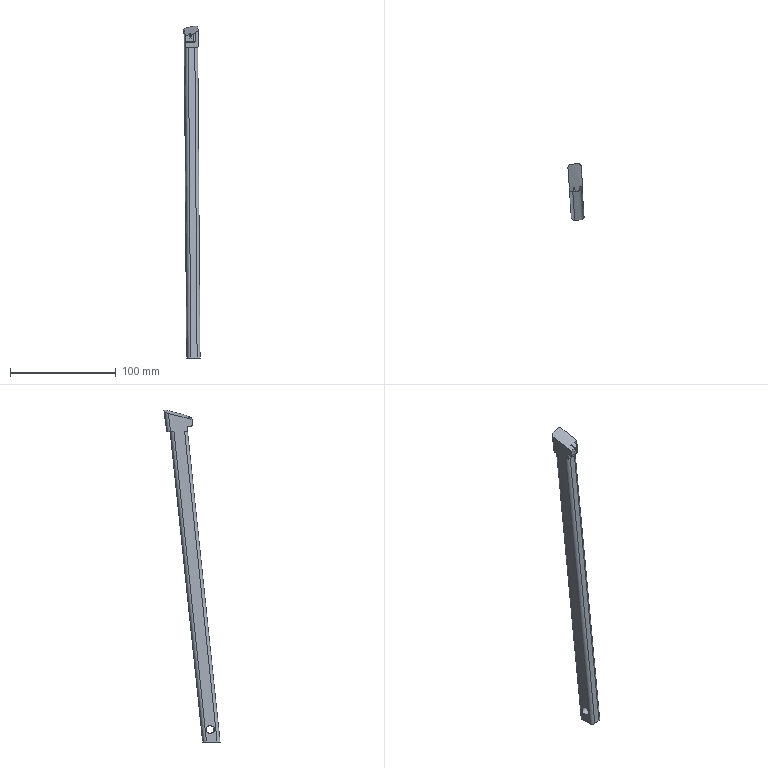Part | STEP file | 车灯-后视镜_id606_x_t | 1 solid | 31 faces | box 15.208 x 52.995 x 313.531 mm | volume 58140 mm3 | plane 19 | cylinder 8 | spline 4 | commonest cylinder face diameters 6 x6 1.018 x1 8 x1